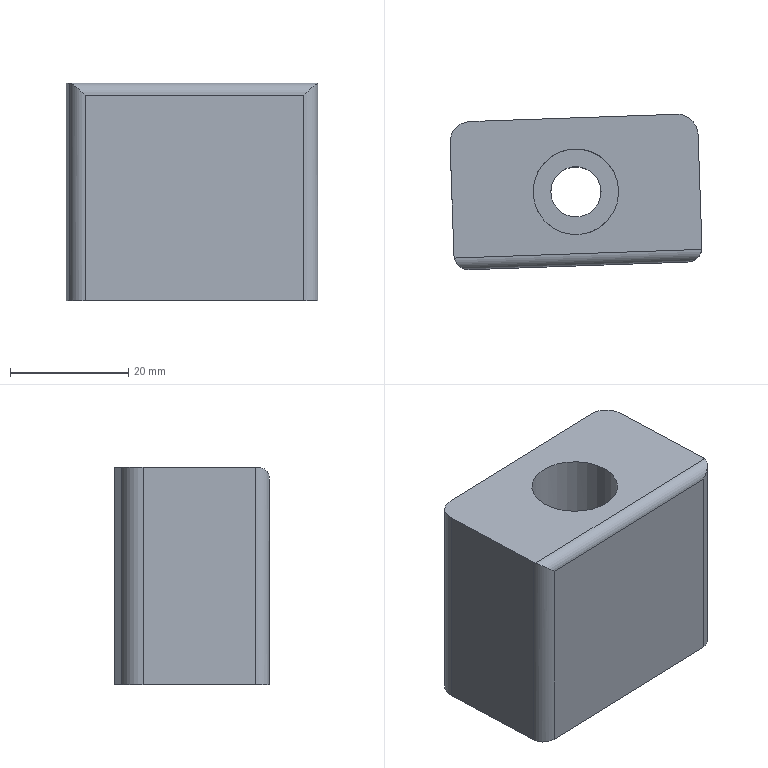Part | NX | features DIE-72 2 | 1 solid | 14 faces | box 42.641 x 26.245 x 36.8 mm | volume 34947 mm3 | plane 7 | cylinder 7 | commonest cylinder face diameters 5 x2 7 x2 4 x1 8.5 x1 14.5 x1
STEP:
#1=CARTESIAN_POINT('',(3662.285,-779.688,823.716));
#2=VERTEX_POINT('',#1);
#3=CARTESIAN_POINT('',(3658.035,-779.688,823.716));
#4=DIRECTION('',(0.,0.,1.));
#5=DIRECTION('',(1.,0.,0.));
#6=AXIS2_PLACEMENT_3D('',#3,#4,#5);
#7=CIRCLE('',#6,4.25);
#8=EDGE_CURVE('',#2,#2,#7,.T.);
#9=ORIENTED_EDGE('',*,*,#8,.T.);
#10=EDGE_LOOP('',(#9));
#11=FACE_BOUND('',#10,.T.);
#12=CARTESIAN_POINT('',(3639.983,-792.826,823.716));
#13=VERTEX_POINT('',#12);
#14=CARTESIAN_POINT('',(3676.96,-791.535,823.716));
#15=VERTEX_POINT('',#14);
#16=CARTESIAN_POINT('',(3672.198,-791.701,823.716));
#17=DIRECTION('',(0.9994,0.0349,0.));
#18=VECTOR('',#17,1000.);
#19=LINE('',#16,#18);
#20=EDGE_CURVE('',#13,#15,#19,.T.);
#21=ORIENTED_EDGE('',*,*,#20,.F.);
#22=CARTESIAN_POINT('',(3637.397,-790.415,823.716));
#23=VERTEX_POINT('',#22);
#24=CARTESIAN_POINT('',(3639.896,-790.328,823.716));
#25=DIRECTION('',(0.,0.,1.));
#26=DIRECTION('',(1.,0.,0.));
#27=AXIS2_PLACEMENT_3D('',#24,#25,#26);
#28=CIRCLE('',#27,2.5);
#29=EDGE_CURVE('',#13,#23,#28,.F.);
#30=ORIENTED_EDGE('',*,*,#29,.T.);
#31=CARTESIAN_POINT('',(3636.734,-771.426,823.716));
#32=VERTEX_POINT('',#31);
#33=CARTESIAN_POINT('',(3638.21,-813.679,823.716));
#34=DIRECTION('',(-0.0349,0.9994,0.));
#35=VECTOR('',#34,1000.);
#36=LINE('',#33,#35);
#37=EDGE_CURVE('',#32,#23,#36,.F.);
#38=ORIENTED_EDGE('',*,*,#37,.F.);
#39=CARTESIAN_POINT('',(3640.11,-767.806,823.716));
#40=VERTEX_POINT('',#39);
#41=CARTESIAN_POINT('',(3640.232,-771.304,823.716));
#42=DIRECTION('',(0.,0.,1.));
#43=DIRECTION('',(1.,0.,0.));
#44=AXIS2_PLACEMENT_3D('',#41,#42,#43);
#45=CIRCLE('',#44,3.5);
#46=EDGE_CURVE('',#32,#40,#45,.F.);
#47=ORIENTED_EDGE('',*,*,#46,.T.);
#48=CARTESIAN_POINT('',(3675.089,-766.585,823.716));
#49=VERTEX_POINT('',#48);
#50=CARTESIAN_POINT('',(3671.325,-766.717,823.716));
#51=DIRECTION('',(0.9994,0.0349,0.));
#52=VECTOR('',#51,1000.);
#53=LINE('',#50,#52);
#54=EDGE_CURVE('',#40,#49,#53,.T.);
#55=ORIENTED_EDGE('',*,*,#54,.T.);
#56=CARTESIAN_POINT('',(3678.709,-769.961,823.716));
#57=VERTEX_POINT('',#56);
#58=CARTESIAN_POINT('',(3675.211,-770.083,823.716));
#59=DIRECTION('',(0.,0.,1.));
#60=DIRECTION('',(1.,0.,0.));
#61=AXIS2_PLACEMENT_3D('',#58,#59,#60);
#62=CIRCLE('',#61,3.5);
#63=EDGE_CURVE('',#49,#57,#62,.F.);
#64=ORIENTED_EDGE('',*,*,#63,.T.);
#65=CARTESIAN_POINT('',(3679.372,-788.949,823.716));
#66=VERTEX_POINT('',#65);
#67=CARTESIAN_POINT('',(3681.133,-839.387,823.716));
#68=DIRECTION('',(0.0349,-0.9994,0.));
#69=VECTOR('',#68,1000.);
#70=LINE('',#67,#69);
#71=EDGE_CURVE('',#57,#66,#70,.T.);
#72=ORIENTED_EDGE('',*,*,#71,.T.);
#73=CARTESIAN_POINT('',(3676.873,-789.037,823.716));
#74=DIRECTION('',(0.,0.,1.));
#75=DIRECTION('',(1.,0.,0.));
#76=AXIS2_PLACEMENT_3D('',#73,#74,#75);
#77=CIRCLE('',#76,2.5);
#78=EDGE_CURVE('',#66,#15,#77,.F.);
#79=ORIENTED_EDGE('',*,*,#78,.T.);
#80=EDGE_LOOP('',(#21,#30,#38,#47,#55,#64,#72,#79));
#81=FACE_BOUND('',#80,.T.);
#82=CARTESIAN_POINT('',(3688.707,-839.123,823.716));
#83=DIRECTION('',(0.,0.,1.));
#84=DIRECTION('',(0.,-1.,0.));
#85=AXIS2_PLACEMENT_3D('',#82,#83,#84);
#86=PLANE('',#85);
#87=ADVANCED_FACE('',(#11,#81),#86,.F.);
#88=CARTESIAN_POINT('',(3678.709,-769.961,860.516));
#89=VERTEX_POINT('',#88);
#90=CARTESIAN_POINT('',(3679.372,-788.949,860.516));
#91=VERTEX_POINT('',#90);
#92=CARTESIAN_POINT('',(3679.977,-806.297,860.516));
#93=DIRECTION('',(-0.0349,0.9994,0.));
#94=VECTOR('',#93,1000.);
#95=LINE('',#92,#94);
#96=EDGE_CURVE('',#89,#91,#95,.F.);
#97=ORIENTED_EDGE('',*,*,#96,.T.);
#98=CARTESIAN_POINT('',(3679.372,-788.949,891.507));
#99=DIRECTION('',(0.,0.,1.));
#100=VECTOR('',#99,1000.);
#101=LINE('',#98,#100);
#102=EDGE_CURVE('',#91,#66,#101,.F.);
#103=ORIENTED_EDGE('',*,*,#102,.T.);
#104=ORIENTED_EDGE('',*,*,#71,.F.);
#105=CARTESIAN_POINT('',(3678.709,-769.961,858.716));
#106=DIRECTION('',(0.,0.,-1.));
#107=VECTOR('',#106,1000.);
#108=LINE('',#105,#107);
#109=EDGE_CURVE('',#57,#89,#108,.F.);
#110=ORIENTED_EDGE('',*,*,#109,.T.);
#111=EDGE_LOOP('',(#97,#103,#104,#110));
#112=FACE_BOUND('',#111,.T.);
#113=CARTESIAN_POINT('',(3679.977,-806.297,891.507));
#114=DIRECTION('',(-0.9994,-0.0349,0.));
#115=DIRECTION('',(-0.0349,0.9994,0.));
#116=AXIS2_PLACEMENT_3D('',#113,#114,#115);
#117=PLANE('',#116);
#118=ADVANCED_FACE('',(#112),#117,.F.);
#119=CARTESIAN_POINT('',(3665.285,-779.688,860.516));
#120=VERTEX_POINT('',#119);
#121=CARTESIAN_POINT('',(3658.035,-779.688,860.516));
#122=DIRECTION('',(0.,0.,1.));
#123=DIRECTION('',(1.,0.,0.));
#124=AXIS2_PLACEMENT_3D('',#121,#122,#123);
#125=CIRCLE('',#124,7.25);
#126=EDGE_CURVE('',#120,#120,#125,.F.);
#127=ORIENTED_EDGE('',*,*,#126,.T.);
#128=EDGE_LOOP('',(#127));
#129=FACE_BOUND('',#128,.T.);
#130=CARTESIAN_POINT('',(3636.734,-771.426,860.516));
#131=VERTEX_POINT('',#130);
#132=CARTESIAN_POINT('',(3637.397,-790.415,860.516));
#133=VERTEX_POINT('',#132);
#134=CARTESIAN_POINT('',(3640.484,-878.806,860.516));
#135=DIRECTION('',(0.0349,-0.9994,0.));
#136=VECTOR('',#135,1000.);
#137=LINE('',#134,#136);
#138=EDGE_CURVE('',#131,#133,#137,.T.);
#139=ORIENTED_EDGE('',*,*,#138,.T.);
#140=CARTESIAN_POINT('',(3637.465,-790.913,860.516));
#141=VERTEX_POINT('',#140);
#142=CARTESIAN_POINT('',(3639.896,-790.328,860.516));
#143=DIRECTION('',(0.,0.,1.));
#144=DIRECTION('',(1.,0.,0.));
#145=AXIS2_PLACEMENT_3D('',#142,#143,#144);
#146=CIRCLE('',#145,2.5);
#147=EDGE_CURVE('',#133,#141,#146,.T.);
#148=ORIENTED_EDGE('',*,*,#147,.T.);
#149=CARTESIAN_POINT('',(3679.339,-789.451,860.516));
#150=VERTEX_POINT('',#149);
#151=CARTESIAN_POINT('',(3685.638,-789.231,860.516));
#152=DIRECTION('',(-0.9994,-0.0349,0.));
#153=VECTOR('',#152,1000.);
#154=LINE('',#151,#153);
#155=EDGE_CURVE('',#150,#141,#154,.T.);
#156=ORIENTED_EDGE('',*,*,#155,.F.);
#157=CARTESIAN_POINT('',(3676.873,-789.037,860.516));
#158=DIRECTION('',(0.,0.,1.));
#159=DIRECTION('',(1.,0.,0.));
#160=AXIS2_PLACEMENT_3D('',#157,#158,#159);
#161=CIRCLE('',#160,2.5);
#162=EDGE_CURVE('',#150,#91,#161,.T.);
#163=ORIENTED_EDGE('',*,*,#162,.T.);
#164=ORIENTED_EDGE('',*,*,#96,.F.);
#165=CARTESIAN_POINT('',(3675.089,-766.585,860.516));
#166=VERTEX_POINT('',#165);
#167=CARTESIAN_POINT('',(3675.211,-770.083,860.516));
#168=DIRECTION('',(0.,0.,1.));
#169=DIRECTION('',(1.,0.,0.));
#170=AXIS2_PLACEMENT_3D('',#167,#168,#169);
#171=CIRCLE('',#170,3.5);
#172=EDGE_CURVE('',#89,#166,#171,.T.);
#173=ORIENTED_EDGE('',*,*,#172,.T.);
#174=CARTESIAN_POINT('',(3640.11,-767.806,860.516));
#175=VERTEX_POINT('',#174);
#176=CARTESIAN_POINT('',(3671.325,-766.717,860.516));
#177=DIRECTION('',(0.9994,0.0349,0.));
#178=VECTOR('',#177,1000.);
#179=LINE('',#176,#178);
#180=EDGE_CURVE('',#166,#175,#179,.F.);
#181=ORIENTED_EDGE('',*,*,#180,.T.);
#182=CARTESIAN_POINT('',(3640.232,-771.304,860.516));
#183=DIRECTION('',(0.,0.,1.));
#184=DIRECTION('',(1.,0.,0.));
#185=AXIS2_PLACEMENT_3D('',#182,#183,#184);
#186=CIRCLE('',#185,3.5);
#187=EDGE_CURVE('',#175,#131,#186,.T.);
#188=ORIENTED_EDGE('',*,*,#187,.T.);
#189=EDGE_LOOP('',(#139,#148,#156,#163,#164,#173,#181,#188));
#190=FACE_BOUND('',#189,.T.);
#191=CARTESIAN_POINT('',(3688.707,-877.122,860.516));
#192=DIRECTION('',(0.,0.,1.));
#193=DIRECTION('',(0.,1.,0.));
#194=AXIS2_PLACEMENT_3D('',#191,#192,#193);
#195=PLANE('',#194);
#196=ADVANCED_FACE('',(#129,#190),#195,.T.);
#197=ORIENTED_EDGE('',*,*,#37,.T.);
#198=CARTESIAN_POINT('',(3637.397,-790.415,948.075));
#199=DIRECTION('',(0.,0.,1.));
#200=VECTOR('',#199,1000.);
#201=LINE('',#198,#200);
#202=EDGE_CURVE('',#23,#133,#201,.T.);
#203=ORIENTED_EDGE('',*,*,#202,.T.);
#204=ORIENTED_EDGE('',*,*,#138,.F.);
#205=CARTESIAN_POINT('',(3636.734,-771.426,823.716));
#206=DIRECTION('',(0.,0.,1.));
#207=VECTOR('',#206,1000.);
#208=LINE('',#205,#207);
#209=EDGE_CURVE('',#131,#32,#208,.F.);
#210=ORIENTED_EDGE('',*,*,#209,.T.);
#211=EDGE_LOOP('',(#197,#203,#204,#210));
#212=FACE_BOUND('',#211,.T.);
#213=CARTESIAN_POINT('',(3638.21,-813.679,948.075));
#214=DIRECTION('',(-0.9994,-0.0349,0.));
#215=DIRECTION('',(-0.0349,0.9994,0.));
#216=AXIS2_PLACEMENT_3D('',#213,#214,#215);
#217=PLANE('',#216);
#218=ADVANCED_FACE('',(#212),#217,.T.);
#219=ORIENTED_EDGE('',*,*,#180,.F.);
#220=CARTESIAN_POINT('',(3675.089,-766.585,823.716));
#221=DIRECTION('',(0.,0.,-1.));
#222=VECTOR('',#221,1000.);
#223=LINE('',#220,#222);
#224=EDGE_CURVE('',#166,#49,#223,.T.);
#225=ORIENTED_EDGE('',*,*,#224,.T.);
#226=ORIENTED_EDGE('',*,*,#54,.F.);
#227=CARTESIAN_POINT('',(3640.11,-767.806,858.716));
#228=DIRECTION('',(0.,0.,-1.));
#229=VECTOR('',#228,1000.);
#230=LINE('',#227,#229);
#231=EDGE_CURVE('',#40,#175,#230,.F.);
#232=ORIENTED_EDGE('',*,*,#231,.T.);
#233=EDGE_LOOP('',(#219,#225,#226,#232));
#234=FACE_BOUND('',#233,.T.);
#235=CARTESIAN_POINT('',(3671.325,-766.717,940.297));
#236=DIRECTION('',(-0.0349,0.9994,0.));
#237=DIRECTION('',(0.9994,0.0349,0.));
#238=AXIS2_PLACEMENT_3D('',#235,#236,#237);
#239=PLANE('',#238);
#240=ADVANCED_FACE('',(#234),#239,.T.);
#241=CARTESIAN_POINT('',(3639.983,-792.826,858.516));
#242=VERTEX_POINT('',#241);
#243=CARTESIAN_POINT('',(3676.96,-791.535,858.516));
#244=VERTEX_POINT('',#243);
#245=CARTESIAN_POINT('',(3685.708,-791.23,858.516));
#246=DIRECTION('',(0.9994,0.0349,0.));
#247=VECTOR('',#246,1000.);
#248=LINE('',#245,#247);
#249=EDGE_CURVE('',#242,#244,#248,.T.);
#250=ORIENTED_EDGE('',*,*,#249,.F.);
#251=CARTESIAN_POINT('',(3639.983,-792.826,940.297));
#252=DIRECTION('',(0.,0.,-1.));
#253=VECTOR('',#252,1000.);
#254=LINE('',#251,#253);
#255=EDGE_CURVE('',#242,#13,#254,.T.);
#256=ORIENTED_EDGE('',*,*,#255,.T.);
#257=ORIENTED_EDGE('',*,*,#20,.T.);
#258=CARTESIAN_POINT('',(3676.96,-791.535,940.297));
#259=DIRECTION('',(0.,0.,1.));
#260=VECTOR('',#259,1000.);
#261=LINE('',#258,#260);
#262=EDGE_CURVE('',#15,#244,#261,.T.);
#263=ORIENTED_EDGE('',*,*,#262,.T.);
#264=EDGE_LOOP('',(#250,#256,#257,#263));
#265=FACE_BOUND('',#264,.T.);
#266=CARTESIAN_POINT('',(3672.198,-791.701,940.297));
#267=DIRECTION('',(-0.0349,0.9994,0.));
#268=DIRECTION('',(0.9994,0.0349,0.));
#269=AXIS2_PLACEMENT_3D('',#266,#267,#268);
#270=PLANE('',#269);
#271=ADVANCED_FACE('',(#265),#270,.F.);
#272=ORIENTED_EDGE('',*,*,#155,.T.);
#273=CARTESIAN_POINT('',(3637.465,-790.913,860.516));
#274=CARTESIAN_POINT('',(3637.625,-791.578,860.516));
#275=CARTESIAN_POINT('',(3638.462,-792.603,859.869));
#276=CARTESIAN_POINT('',(3639.482,-792.844,858.965));
#277=CARTESIAN_POINT('',(3639.983,-792.826,858.516));
#278=B_SPLINE_CURVE_WITH_KNOTS('',3,(#273,#274,#275,#276,#277),.UNSPECIFIED.,.F.,.F.,(4,1,4),(0.,0.002017,0.004035),.UNSPECIFIED.);
#279=EDGE_CURVE('',#141,#242,#278,.T.);
#280=ORIENTED_EDGE('',*,*,#279,.T.);
#281=ORIENTED_EDGE('',*,*,#249,.T.);
#282=CARTESIAN_POINT('',(3679.339,-789.451,860.516));
#283=CARTESIAN_POINT('',(3679.225,-790.126,860.516));
#284=CARTESIAN_POINT('',(3678.462,-791.207,859.869));
#285=CARTESIAN_POINT('',(3677.461,-791.518,858.965));
#286=CARTESIAN_POINT('',(3676.96,-791.535,858.516));
#287=B_SPLINE_CURVE_WITH_KNOTS('',3,(#282,#283,#284,#285,#286),.UNSPECIFIED.,.F.,.F.,(4,1,4),(0.,0.002017,0.004035),.UNSPECIFIED.);
#288=EDGE_CURVE('',#244,#150,#287,.F.);
#289=ORIENTED_EDGE('',*,*,#288,.T.);
#290=EDGE_LOOP('',(#272,#280,#281,#289));
#291=FACE_BOUND('',#290,.T.);
#292=CARTESIAN_POINT('',(3685.638,-789.231,858.516));
#293=DIRECTION('',(-0.9994,-0.0349,0.));
#294=DIRECTION('',(0.0349,-0.9994,0.));
#295=AXIS2_PLACEMENT_3D('',#292,#293,#294);
#296=CYLINDRICAL_SURFACE('',#295,2.);
#297=ADVANCED_FACE('',(#291),#296,.T.);
#298=ORIENTED_EDGE('',*,*,#172,.F.);
#299=ORIENTED_EDGE('',*,*,#109,.F.);
#300=ORIENTED_EDGE('',*,*,#63,.F.);
#301=ORIENTED_EDGE('',*,*,#224,.F.);
#302=EDGE_LOOP('',(#298,#299,#300,#301));
#303=FACE_BOUND('',#302,.T.);
#304=CARTESIAN_POINT('',(3675.211,-770.083,940.297));
#305=DIRECTION('',(0.,0.,1.));
#306=DIRECTION('',(1.,0.,0.));
#307=AXIS2_PLACEMENT_3D('',#304,#305,#306);
#308=CYLINDRICAL_SURFACE('',#307,3.5);
#309=ADVANCED_FACE('',(#303),#308,.T.);
#310=ORIENTED_EDGE('',*,*,#46,.F.);
#311=ORIENTED_EDGE('',*,*,#209,.F.);
#312=ORIENTED_EDGE('',*,*,#187,.F.);
#313=ORIENTED_EDGE('',*,*,#231,.F.);
#314=EDGE_LOOP('',(#310,#311,#312,#313));
#315=FACE_BOUND('',#314,.T.);
#316=CARTESIAN_POINT('',(3640.232,-771.304,940.297));
#317=DIRECTION('',(0.,0.,1.));
#318=DIRECTION('',(1.,0.,0.));
#319=AXIS2_PLACEMENT_3D('',#316,#317,#318);
#320=CYLINDRICAL_SURFACE('',#319,3.5);
#321=ADVANCED_FACE('',(#315),#320,.T.);
#322=ORIENTED_EDGE('',*,*,#29,.F.);
#323=ORIENTED_EDGE('',*,*,#255,.F.);
#324=ORIENTED_EDGE('',*,*,#279,.F.);
#325=ORIENTED_EDGE('',*,*,#147,.F.);
#326=ORIENTED_EDGE('',*,*,#202,.F.);
#327=EDGE_LOOP('',(#322,#323,#324,#325,#326));
#328=FACE_BOUND('',#327,.T.);
#329=CARTESIAN_POINT('',(3639.896,-790.328,948.075));
#330=DIRECTION('',(0.,0.,-1.));
#331=DIRECTION('',(-1.,0.,0.));
#332=AXIS2_PLACEMENT_3D('',#329,#330,#331);
#333=CYLINDRICAL_SURFACE('',#332,2.5);
#334=ADVANCED_FACE('',(#328),#333,.T.);
#335=ORIENTED_EDGE('',*,*,#78,.F.);
#336=ORIENTED_EDGE('',*,*,#102,.F.);
#337=ORIENTED_EDGE('',*,*,#162,.F.);
#338=ORIENTED_EDGE('',*,*,#288,.F.);
#339=ORIENTED_EDGE('',*,*,#262,.F.);
#340=EDGE_LOOP('',(#335,#336,#337,#338,#339));
#341=FACE_BOUND('',#340,.T.);
#342=CARTESIAN_POINT('',(3676.873,-789.037,940.297));
#343=DIRECTION('',(0.,0.,1.));
#344=DIRECTION('',(1.,0.,0.));
#345=AXIS2_PLACEMENT_3D('',#342,#343,#344);
#346=CYLINDRICAL_SURFACE('',#345,2.5);
#347=ADVANCED_FACE('',(#341),#346,.T.);
#348=CARTESIAN_POINT('',(3662.285,-779.688,848.716));
#349=VERTEX_POINT('',#348);
#350=CARTESIAN_POINT('',(3658.035,-779.688,848.716));
#351=DIRECTION('',(0.,0.,1.));
#352=DIRECTION('',(1.,0.,0.));
#353=AXIS2_PLACEMENT_3D('',#350,#351,#352);
#354=CIRCLE('',#353,4.25);
#355=EDGE_CURVE('',#349,#349,#354,.T.);
#356=ORIENTED_EDGE('',*,*,#355,.T.);
#357=EDGE_LOOP('',(#356));
#358=FACE_BOUND('',#357,.T.);
#359=ORIENTED_EDGE('',*,*,#8,.F.);
#360=EDGE_LOOP('',(#359));
#361=FACE_BOUND('',#360,.T.);
#362=CARTESIAN_POINT('',(3658.035,-779.688,822.716));
#363=DIRECTION('',(0.,0.,1.));
#364=DIRECTION('',(1.,0.,0.));
#365=AXIS2_PLACEMENT_3D('',#362,#363,#364);
#366=CYLINDRICAL_SURFACE('',#365,4.25);
#367=ADVANCED_FACE('',(#358,#361),#366,.F.);
#368=CARTESIAN_POINT('',(3650.79,-779.941,848.716));
#369=VERTEX_POINT('',#368);
#370=CARTESIAN_POINT('',(3658.035,-779.688,848.716));
#371=DIRECTION('',(0.,0.,1.));
#372=DIRECTION('',(-0.9994,-0.0349,0.));
#373=AXIS2_PLACEMENT_3D('',#370,#371,#372);
#374=CIRCLE('',#373,7.25);
#375=EDGE_CURVE('',#369,#369,#374,.F.);
#376=ORIENTED_EDGE('',*,*,#375,.T.);
#377=EDGE_LOOP('',(#376));
#378=FACE_BOUND('',#377,.T.);
#379=ORIENTED_EDGE('',*,*,#126,.F.);
#380=EDGE_LOOP('',(#379));
#381=FACE_BOUND('',#380,.T.);
#382=CARTESIAN_POINT('',(3658.035,-779.688,848.716));
#383=DIRECTION('',(0.,0.,1.));
#384=DIRECTION('',(1.,0.,0.));
#385=AXIS2_PLACEMENT_3D('',#382,#383,#384);
#386=CYLINDRICAL_SURFACE('',#385,7.25);
#387=ADVANCED_FACE('',(#378,#381),#386,.F.);
#388=ORIENTED_EDGE('',*,*,#355,.F.);
#389=EDGE_LOOP('',(#388));
#390=FACE_BOUND('',#389,.T.);
#391=ORIENTED_EDGE('',*,*,#375,.F.);
#392=EDGE_LOOP('',(#391));
#393=FACE_BOUND('',#392,.T.);
#394=CARTESIAN_POINT('',(3658.035,-779.688,848.716));
#395=DIRECTION('',(0.,0.,1.));
#396=DIRECTION('',(1.,0.,0.));
#397=AXIS2_PLACEMENT_3D('',#394,#395,#396);
#398=PLANE('',#397);
#399=ADVANCED_FACE('',(#390,#393),#398,.T.);
#400=CLOSED_SHELL('',(#87,#118,#196,#218,#240,#271,#297,#309,#321,#334,#347,#367,#387,#399));
#401=MANIFOLD_SOLID_BREP('',#400);
#402=(LENGTH_UNIT()NAMED_UNIT(*)SI_UNIT(.MILLI.,.METRE.));
#403=UNCERTAINTY_MEASURE_WITH_UNIT(LENGTH_MEASURE(0.0508),#402,'','');
#404=(NAMED_UNIT(*)PLANE_ANGLE_UNIT()SI_UNIT($,.RADIAN.));
#405=(NAMED_UNIT(*)SI_UNIT($,.STERADIAN.)SOLID_ANGLE_UNIT());
#406=(GEOMETRIC_REPRESENTATION_CONTEXT(3)GLOBAL_UNCERTAINTY_ASSIGNED_CONTEXT((#403))GLOBAL_UNIT_ASSIGNED_CONTEXT((#402,#404,#405))REPRESENTATION_CONTEXT('',''));
#407=ADVANCED_BREP_SHAPE_REPRESENTATION('',(#401),#406);